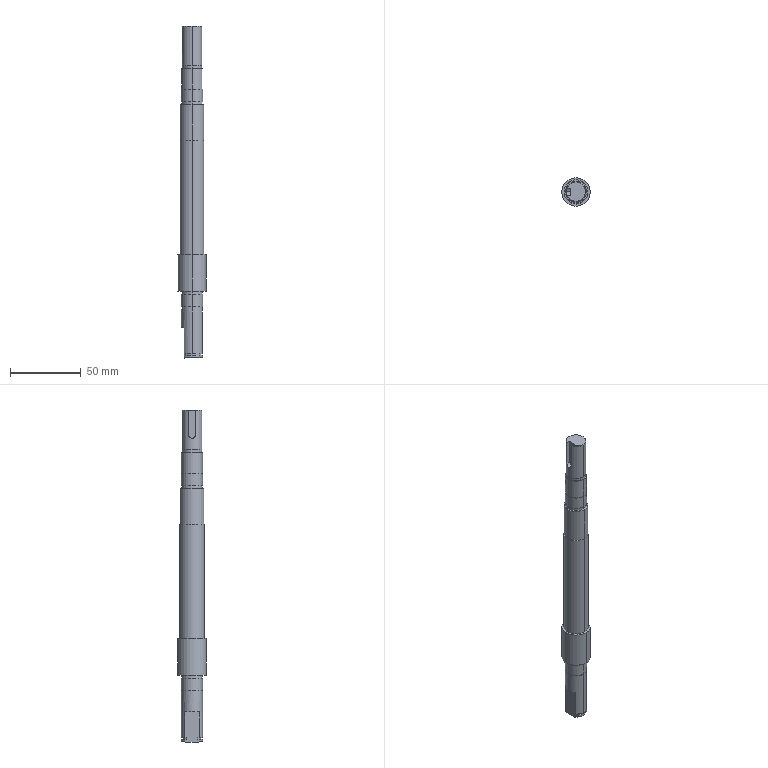Part | SolidWorks | features BaseBody 1 | 1 solid | 54 faces | box 20 x 20 x 234 mm | volume 48637 mm3 | cylinder 30 | plane 19 | cone 5 | commonest cylinder face diameters 14.9 x7 14.6 x4 15 x4 13.3 x3 5 x2 13.6 x2